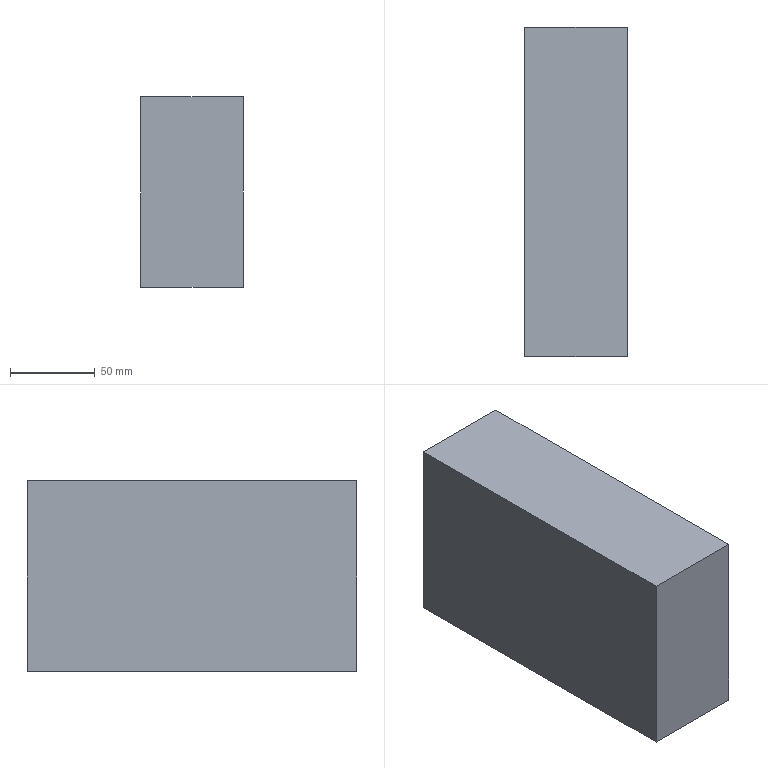Part | SolidWorks | features BaseBody 1 | 1 solid | 6 faces | box 60.7 x 194.65 x 112.8 mm | volume 1332761 mm3 | plane 6
STEP:
#1=CARTESIAN_POINT('',(-472.128,-87.33,2.5));
#2=VERTEX_POINT('',#1);
#3=CARTESIAN_POINT('',(-472.128,107.32,2.5));
#4=VERTEX_POINT('',#3);
#5=CARTESIAN_POINT('',(-472.128,9.995,2.5));
#6=DIRECTION('',(0.,1.,0.));
#7=VECTOR('',#6,1000.);
#8=LINE('',#5,#7);
#9=EDGE_CURVE('',#2,#4,#8,.T.);
#10=ORIENTED_EDGE('',*,*,#9,.T.);
#11=CARTESIAN_POINT('',(-472.128,107.32,115.3));
#12=VERTEX_POINT('',#11);
#13=CARTESIAN_POINT('',(-472.128,107.32,58.9));
#14=DIRECTION('',(0.,0.,1.));
#15=VECTOR('',#14,1000.);
#16=LINE('',#13,#15);
#17=EDGE_CURVE('',#4,#12,#16,.T.);
#18=ORIENTED_EDGE('',*,*,#17,.T.);
#19=CARTESIAN_POINT('',(-472.128,-87.33,115.3));
#20=VERTEX_POINT('',#19);
#21=CARTESIAN_POINT('',(-472.128,9.995,115.3));
#22=DIRECTION('',(0.,-1.,0.));
#23=VECTOR('',#22,1000.);
#24=LINE('',#21,#23);
#25=EDGE_CURVE('',#12,#20,#24,.T.);
#26=ORIENTED_EDGE('',*,*,#25,.T.);
#27=CARTESIAN_POINT('',(-472.128,-87.33,58.9));
#28=DIRECTION('',(0.,0.,-1.));
#29=VECTOR('',#28,1000.);
#30=LINE('',#27,#29);
#31=EDGE_CURVE('',#20,#2,#30,.T.);
#32=ORIENTED_EDGE('',*,*,#31,.T.);
#33=EDGE_LOOP('',(#10,#18,#26,#32));
#34=FACE_OUTER_BOUND('',#33,.T.);
#35=CARTESIAN_POINT('',(-472.128,9.995,58.9));
#36=DIRECTION('',(1.,0.,0.));
#37=DIRECTION('',(0.,0.,-1.));
#38=AXIS2_PLACEMENT_3D('',#35,#36,#37);
#39=PLANE('',#38);
#40=ADVANCED_FACE('',(#34),#39,.T.);
#41=CARTESIAN_POINT('',(-532.828,107.32,2.5));
#42=VERTEX_POINT('',#41);
#43=CARTESIAN_POINT('',(-502.478,107.32,2.5));
#44=DIRECTION('',(-1.,0.,0.));
#45=VECTOR('',#44,1000.);
#46=LINE('',#43,#45);
#47=EDGE_CURVE('',#4,#42,#46,.T.);
#48=ORIENTED_EDGE('',*,*,#47,.T.);
#49=CARTESIAN_POINT('',(-532.828,107.32,115.3));
#50=VERTEX_POINT('',#49);
#51=CARTESIAN_POINT('',(-532.828,107.32,58.9));
#52=DIRECTION('',(0.,0.,1.));
#53=VECTOR('',#52,1000.);
#54=LINE('',#51,#53);
#55=EDGE_CURVE('',#42,#50,#54,.T.);
#56=ORIENTED_EDGE('',*,*,#55,.T.);
#57=CARTESIAN_POINT('',(-502.478,107.32,115.3));
#58=DIRECTION('',(1.,0.,0.));
#59=VECTOR('',#58,1000.);
#60=LINE('',#57,#59);
#61=EDGE_CURVE('',#50,#12,#60,.T.);
#62=ORIENTED_EDGE('',*,*,#61,.T.);
#63=ORIENTED_EDGE('',*,*,#17,.F.);
#64=EDGE_LOOP('',(#48,#56,#62,#63));
#65=FACE_OUTER_BOUND('',#64,.T.);
#66=CARTESIAN_POINT('',(-502.478,107.32,58.9));
#67=DIRECTION('',(0.,1.,0.));
#68=DIRECTION('',(-1.,0.,0.));
#69=AXIS2_PLACEMENT_3D('',#66,#67,#68);
#70=PLANE('',#69);
#71=ADVANCED_FACE('',(#65),#70,.T.);
#72=ORIENTED_EDGE('',*,*,#9,.F.);
#73=CARTESIAN_POINT('',(-532.828,-87.33,2.5));
#74=VERTEX_POINT('',#73);
#75=CARTESIAN_POINT('',(-502.478,-87.33,2.5));
#76=DIRECTION('',(-1.,0.,0.));
#77=VECTOR('',#76,1000.);
#78=LINE('',#75,#77);
#79=EDGE_CURVE('',#2,#74,#78,.T.);
#80=ORIENTED_EDGE('',*,*,#79,.T.);
#81=CARTESIAN_POINT('',(-532.828,9.995,2.5));
#82=DIRECTION('',(0.,1.,0.));
#83=VECTOR('',#82,1000.);
#84=LINE('',#81,#83);
#85=EDGE_CURVE('',#74,#42,#84,.T.);
#86=ORIENTED_EDGE('',*,*,#85,.T.);
#87=ORIENTED_EDGE('',*,*,#47,.F.);
#88=EDGE_LOOP('',(#72,#80,#86,#87));
#89=FACE_OUTER_BOUND('',#88,.T.);
#90=CARTESIAN_POINT('',(-502.478,9.995,2.5));
#91=DIRECTION('',(0.,0.,-1.));
#92=DIRECTION('',(-1.,0.,0.));
#93=AXIS2_PLACEMENT_3D('',#90,#91,#92);
#94=PLANE('',#93);
#95=ADVANCED_FACE('',(#89),#94,.T.);
#96=ORIENTED_EDGE('',*,*,#79,.F.);
#97=ORIENTED_EDGE('',*,*,#31,.F.);
#98=CARTESIAN_POINT('',(-532.828,-87.33,115.3));
#99=VERTEX_POINT('',#98);
#100=CARTESIAN_POINT('',(-502.478,-87.33,115.3));
#101=DIRECTION('',(-1.,0.,0.));
#102=VECTOR('',#101,1000.);
#103=LINE('',#100,#102);
#104=EDGE_CURVE('',#20,#99,#103,.T.);
#105=ORIENTED_EDGE('',*,*,#104,.T.);
#106=CARTESIAN_POINT('',(-532.828,-87.33,58.9));
#107=DIRECTION('',(0.,0.,-1.));
#108=VECTOR('',#107,1000.);
#109=LINE('',#106,#108);
#110=EDGE_CURVE('',#99,#74,#109,.T.);
#111=ORIENTED_EDGE('',*,*,#110,.T.);
#112=EDGE_LOOP('',(#96,#97,#105,#111));
#113=FACE_OUTER_BOUND('',#112,.T.);
#114=CARTESIAN_POINT('',(-502.478,-87.33,58.9));
#115=DIRECTION('',(0.,-1.,0.));
#116=DIRECTION('',(1.,0.,0.));
#117=AXIS2_PLACEMENT_3D('',#114,#115,#116);
#118=PLANE('',#117);
#119=ADVANCED_FACE('',(#113),#118,.T.);
#120=ORIENTED_EDGE('',*,*,#25,.F.);
#121=ORIENTED_EDGE('',*,*,#61,.F.);
#122=CARTESIAN_POINT('',(-532.828,9.995,115.3));
#123=DIRECTION('',(0.,-1.,0.));
#124=VECTOR('',#123,1000.);
#125=LINE('',#122,#124);
#126=EDGE_CURVE('',#50,#99,#125,.T.);
#127=ORIENTED_EDGE('',*,*,#126,.T.);
#128=ORIENTED_EDGE('',*,*,#104,.F.);
#129=EDGE_LOOP('',(#120,#121,#127,#128));
#130=FACE_OUTER_BOUND('',#129,.T.);
#131=CARTESIAN_POINT('',(-502.478,9.995,115.3));
#132=DIRECTION('',(0.,0.,1.));
#133=DIRECTION('',(1.,0.,0.));
#134=AXIS2_PLACEMENT_3D('',#131,#132,#133);
#135=PLANE('',#134);
#136=ADVANCED_FACE('',(#130),#135,.T.);
#137=ORIENTED_EDGE('',*,*,#85,.F.);
#138=ORIENTED_EDGE('',*,*,#110,.F.);
#139=ORIENTED_EDGE('',*,*,#126,.F.);
#140=ORIENTED_EDGE('',*,*,#55,.F.);
#141=EDGE_LOOP('',(#137,#138,#139,#140));
#142=FACE_OUTER_BOUND('',#141,.T.);
#143=CARTESIAN_POINT('',(-532.828,9.995,58.9));
#144=DIRECTION('',(-1.,0.,0.));
#145=DIRECTION('',(0.,0.,1.));
#146=AXIS2_PLACEMENT_3D('',#143,#144,#145);
#147=PLANE('',#146);
#148=ADVANCED_FACE('',(#142),#147,.T.);
#149=CLOSED_SHELL('',(#40,#71,#95,#119,#136,#148));
#150=MANIFOLD_SOLID_BREP('',#149);
#151=CARTESIAN_POINT('',(0.,0.,0.));
#152=DIRECTION('',(0.,0.,1.));
#153=DIRECTION('',(1.,0.,0.));
#154=AXIS2_PLACEMENT_3D('',#151,#152,#153);
#155=(LENGTH_UNIT()NAMED_UNIT(*)SI_UNIT(.MILLI.,.METRE.));
#156=UNCERTAINTY_MEASURE_WITH_UNIT(LENGTH_MEASURE(0.00001),#155,'','');
#157=(NAMED_UNIT(*)PLANE_ANGLE_UNIT()SI_UNIT($,.RADIAN.));
#158=(NAMED_UNIT(*)SI_UNIT($,.STERADIAN.)SOLID_ANGLE_UNIT());
#159=(GEOMETRIC_REPRESENTATION_CONTEXT(3)GLOBAL_UNCERTAINTY_ASSIGNED_CONTEXT((#156))GLOBAL_UNIT_ASSIGNED_CONTEXT((#155,#157,#158))REPRESENTATION_CONTEXT('',''));
#160=ADVANCED_BREP_SHAPE_REPRESENTATION('',(#150,#154),#159);